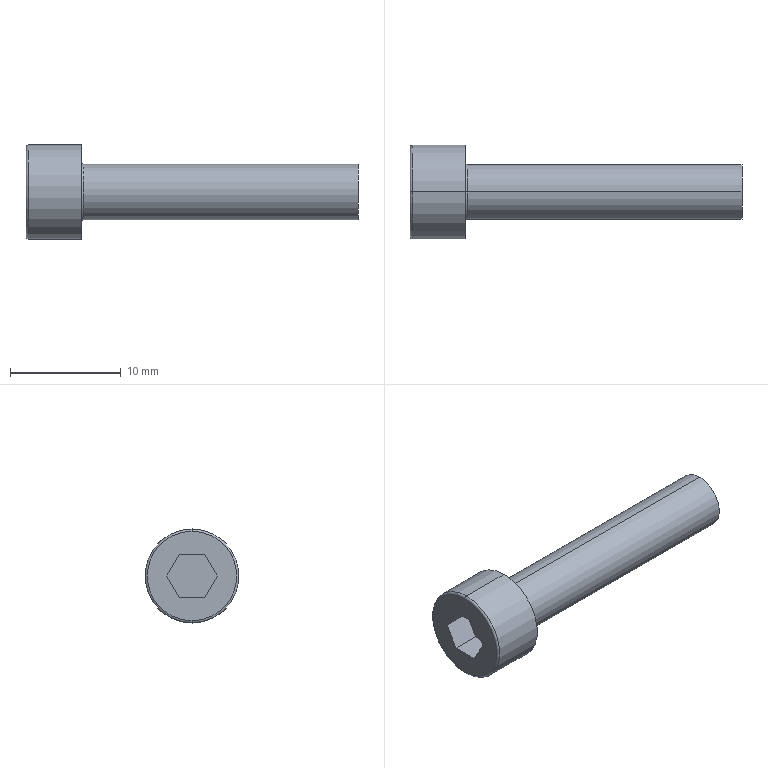Part | SolidWorks | features BlendCut 1, Cut 1, Fillet 1, LPattern 1, RevCut 1, Revolution 1 | 1 solid | 18 faces | box 30 x 8.5 x 8.5 mm | volume 740.448 mm3 | plane 10 | torus 4 | cylinder 4 | commonest cylinder face diameters 5 x2 8.5 x2
STEP:
#1=CARTESIAN_POINT('',(0.2,0.,-4.25));
#2=VERTEX_POINT('',#1);
#3=CARTESIAN_POINT('',(0.2,0.,4.25));
#4=VERTEX_POINT('',#3);
#5=CARTESIAN_POINT('',(0.2,0.,0.));
#6=DIRECTION('',(1.,0.,0.));
#7=DIRECTION('',(0.,0.,1.));
#8=AXIS2_PLACEMENT_3D('',#5,#6,#7);
#9=CIRCLE('',#8,4.25);
#10=EDGE_CURVE('',#2,#4,#9,.T.);
#11=ORIENTED_EDGE('',*,*,#10,.F.);
#12=CARTESIAN_POINT('',(0.,0.,-4.05));
#13=VERTEX_POINT('',#12);
#14=CARTESIAN_POINT('',(0.2,0.,-4.05));
#15=DIRECTION('',(0.,1.,0.));
#16=DIRECTION('',(0.,0.,1.));
#17=AXIS2_PLACEMENT_3D('',#14,#15,#16);
#18=CIRCLE('',#17,0.2);
#19=EDGE_CURVE('',#2,#13,#18,.T.);
#20=ORIENTED_EDGE('',*,*,#19,.T.);
#21=CARTESIAN_POINT('',(0.,0.,4.05));
#22=VERTEX_POINT('',#21);
#23=CARTESIAN_POINT('',(0.,0.,0.));
#24=DIRECTION('',(-1.,0.,0.));
#25=DIRECTION('',(0.,0.,1.));
#26=AXIS2_PLACEMENT_3D('',#23,#24,#25);
#27=CIRCLE('',#26,4.05);
#28=EDGE_CURVE('',#22,#13,#27,.T.);
#29=ORIENTED_EDGE('',*,*,#28,.F.);
#30=CARTESIAN_POINT('',(0.2,0.,4.05));
#31=DIRECTION('',(0.,-1.,0.));
#32=DIRECTION('',(0.,0.,-1.));
#33=AXIS2_PLACEMENT_3D('',#30,#31,#32);
#34=CIRCLE('',#33,0.2);
#35=EDGE_CURVE('',#4,#22,#34,.T.);
#36=ORIENTED_EDGE('',*,*,#35,.F.);
#37=EDGE_LOOP('',(#11,#20,#29,#36));
#38=FACE_OUTER_BOUND('',#37,.T.);
#39=CARTESIAN_POINT('',(0.2,0.,0.));
#40=DIRECTION('',(-1.,0.,0.));
#41=DIRECTION('',(0.,0.,1.));
#42=AXIS2_PLACEMENT_3D('',#39,#40,#41);
#43=TOROIDAL_SURFACE('',#42,4.05,0.2);
#44=ADVANCED_FACE('',(#38),#43,.T.);
#45=CARTESIAN_POINT('',(5.2,0.,-2.5));
#46=VERTEX_POINT('',#45);
#47=CARTESIAN_POINT('',(5.2,0.,2.5));
#48=VERTEX_POINT('',#47);
#49=CARTESIAN_POINT('',(5.2,0.,0.));
#50=DIRECTION('',(1.,0.,0.));
#51=DIRECTION('',(0.,0.,-1.));
#52=AXIS2_PLACEMENT_3D('',#49,#50,#51);
#53=CIRCLE('',#52,2.5);
#54=EDGE_CURVE('',#46,#48,#53,.T.);
#55=ORIENTED_EDGE('',*,*,#54,.T.);
#56=CARTESIAN_POINT('',(30.,0.,2.5));
#57=VERTEX_POINT('',#56);
#58=CARTESIAN_POINT('',(0.,0.,2.5));
#59=DIRECTION('',(1.,0.,0.));
#60=VECTOR('',#59,1000.);
#61=LINE('',#58,#60);
#62=EDGE_CURVE('',#48,#57,#61,.T.);
#63=ORIENTED_EDGE('',*,*,#62,.T.);
#64=CARTESIAN_POINT('',(30.,0.,-2.5));
#65=VERTEX_POINT('',#64);
#66=CARTESIAN_POINT('',(30.,0.,0.));
#67=DIRECTION('',(1.,0.,0.));
#68=DIRECTION('',(0.,0.,-1.));
#69=AXIS2_PLACEMENT_3D('',#66,#67,#68);
#70=CIRCLE('',#69,2.5);
#71=EDGE_CURVE('',#65,#57,#70,.T.);
#72=ORIENTED_EDGE('',*,*,#71,.F.);
#73=CARTESIAN_POINT('',(0.,0.,-2.5));
#74=DIRECTION('',(1.,0.,0.));
#75=VECTOR('',#74,1000.);
#76=LINE('',#73,#75);
#77=EDGE_CURVE('',#46,#65,#76,.T.);
#78=ORIENTED_EDGE('',*,*,#77,.F.);
#79=EDGE_LOOP('',(#55,#63,#72,#78));
#80=FACE_OUTER_BOUND('',#79,.T.);
#81=CARTESIAN_POINT('',(0.,0.,0.));
#82=DIRECTION('',(1.,0.,0.));
#83=DIRECTION('',(0.,0.,-1.));
#84=AXIS2_PLACEMENT_3D('',#81,#82,#83);
#85=CYLINDRICAL_SURFACE('',#84,2.5);
#86=ADVANCED_FACE('',(#80),#85,.T.);
#87=CARTESIAN_POINT('',(5.2,0.,0.));
#88=DIRECTION('',(1.,0.,0.));
#89=DIRECTION('',(0.,0.,-1.));
#90=AXIS2_PLACEMENT_3D('',#87,#88,#89);
#91=CIRCLE('',#90,2.5);
#92=EDGE_CURVE('',#48,#46,#91,.T.);
#93=ORIENTED_EDGE('',*,*,#92,.F.);
#94=CARTESIAN_POINT('',(5.,0.,2.7));
#95=VERTEX_POINT('',#94);
#96=CARTESIAN_POINT('',(5.2,0.,2.7));
#97=DIRECTION('',(0.,1.,0.));
#98=DIRECTION('',(0.,0.,1.));
#99=AXIS2_PLACEMENT_3D('',#96,#97,#98);
#100=CIRCLE('',#99,0.2);
#101=EDGE_CURVE('',#48,#95,#100,.T.);
#102=ORIENTED_EDGE('',*,*,#101,.T.);
#103=CARTESIAN_POINT('',(5.,0.,-2.7));
#104=VERTEX_POINT('',#103);
#105=CARTESIAN_POINT('',(5.,0.,0.));
#106=DIRECTION('',(1.,0.,0.));
#107=DIRECTION('',(0.,0.,-1.));
#108=AXIS2_PLACEMENT_3D('',#105,#106,#107);
#109=CIRCLE('',#108,2.7);
#110=EDGE_CURVE('',#95,#104,#109,.T.);
#111=ORIENTED_EDGE('',*,*,#110,.T.);
#112=CARTESIAN_POINT('',(5.2,0.,-2.7));
#113=DIRECTION('',(0.,-1.,0.));
#114=DIRECTION('',(0.,0.,-1.));
#115=AXIS2_PLACEMENT_3D('',#112,#113,#114);
#116=CIRCLE('',#115,0.2);
#117=EDGE_CURVE('',#46,#104,#116,.T.);
#118=ORIENTED_EDGE('',*,*,#117,.F.);
#119=EDGE_LOOP('',(#93,#102,#111,#118));
#120=FACE_OUTER_BOUND('',#119,.T.);
#121=CARTESIAN_POINT('',(5.2,0.,0.));
#122=DIRECTION('',(1.,0.,0.));
#123=DIRECTION('',(0.,0.,-1.));
#124=AXIS2_PLACEMENT_3D('',#121,#122,#123);
#125=TOROIDAL_SURFACE('',#124,2.7,0.2);
#126=ADVANCED_FACE('',(#120),#125,.F.);
#127=ORIENTED_EDGE('',*,*,#10,.T.);
#128=CARTESIAN_POINT('',(5.,0.,4.25));
#129=VERTEX_POINT('',#128);
#130=CARTESIAN_POINT('',(0.,0.,4.25));
#131=DIRECTION('',(1.,0.,0.));
#132=VECTOR('',#131,1000.);
#133=LINE('',#130,#132);
#134=EDGE_CURVE('',#4,#129,#133,.T.);
#135=ORIENTED_EDGE('',*,*,#134,.T.);
#136=CARTESIAN_POINT('',(5.,0.,-4.25));
#137=VERTEX_POINT('',#136);
#138=CARTESIAN_POINT('',(5.,0.,0.));
#139=DIRECTION('',(1.,0.,0.));
#140=DIRECTION('',(0.,0.,-1.));
#141=AXIS2_PLACEMENT_3D('',#138,#139,#140);
#142=CIRCLE('',#141,4.25);
#143=EDGE_CURVE('',#137,#129,#142,.T.);
#144=ORIENTED_EDGE('',*,*,#143,.F.);
#145=CARTESIAN_POINT('',(0.,0.,-4.25));
#146=DIRECTION('',(1.,0.,0.));
#147=VECTOR('',#146,1000.);
#148=LINE('',#145,#147);
#149=EDGE_CURVE('',#2,#137,#148,.T.);
#150=ORIENTED_EDGE('',*,*,#149,.F.);
#151=EDGE_LOOP('',(#127,#135,#144,#150));
#152=FACE_OUTER_BOUND('',#151,.T.);
#153=CARTESIAN_POINT('',(0.,0.,0.));
#154=DIRECTION('',(1.,0.,0.));
#155=DIRECTION('',(0.,0.,-1.));
#156=AXIS2_PLACEMENT_3D('',#153,#154,#155);
#157=CYLINDRICAL_SURFACE('',#156,4.25);
#158=ADVANCED_FACE('',(#152),#157,.T.);
#159=ORIENTED_EDGE('',*,*,#28,.T.);
#160=CARTESIAN_POINT('',(0.,0.,0.));
#161=DIRECTION('',(-1.,0.,0.));
#162=DIRECTION('',(0.,0.,1.));
#163=AXIS2_PLACEMENT_3D('',#160,#161,#162);
#164=CIRCLE('',#163,4.05);
#165=EDGE_CURVE('',#13,#22,#164,.T.);
#166=ORIENTED_EDGE('',*,*,#165,.T.);
#167=EDGE_LOOP('',(#159,#166));
#168=FACE_OUTER_BOUND('',#167,.T.);
#169=CARTESIAN_POINT('',(0.,-2.29,0.));
#170=VERTEX_POINT('',#169);
#171=CARTESIAN_POINT('',(0.,-1.145,1.983));
#172=VERTEX_POINT('',#171);
#173=CARTESIAN_POINT('',(0.,-2.29,0.));
#174=DIRECTION('',(0.,0.5,0.866));
#175=VECTOR('',#174,1000.);
#176=LINE('',#173,#175);
#177=EDGE_CURVE('',#170,#172,#176,.T.);
#178=ORIENTED_EDGE('',*,*,#177,.F.);
#179=CARTESIAN_POINT('',(0.,-1.145,-1.983));
#180=VERTEX_POINT('',#179);
#181=CARTESIAN_POINT('',(0.,-1.145,-1.983));
#182=DIRECTION('',(0.,-0.5,0.866));
#183=VECTOR('',#182,1000.);
#184=LINE('',#181,#183);
#185=EDGE_CURVE('',#180,#170,#184,.T.);
#186=ORIENTED_EDGE('',*,*,#185,.F.);
#187=CARTESIAN_POINT('',(0.,1.145,-1.983));
#188=VERTEX_POINT('',#187);
#189=CARTESIAN_POINT('',(0.,1.145,-1.983));
#190=DIRECTION('',(0.,-1.,0.));
#191=VECTOR('',#190,1000.);
#192=LINE('',#189,#191);
#193=EDGE_CURVE('',#188,#180,#192,.T.);
#194=ORIENTED_EDGE('',*,*,#193,.F.);
#195=CARTESIAN_POINT('',(0.,2.29,0.));
#196=VERTEX_POINT('',#195);
#197=CARTESIAN_POINT('',(0.,2.29,0.));
#198=DIRECTION('',(0.,-0.5,-0.866));
#199=VECTOR('',#198,1000.);
#200=LINE('',#197,#199);
#201=EDGE_CURVE('',#196,#188,#200,.T.);
#202=ORIENTED_EDGE('',*,*,#201,.F.);
#203=CARTESIAN_POINT('',(0.,1.145,1.983));
#204=VERTEX_POINT('',#203);
#205=CARTESIAN_POINT('',(0.,1.145,1.983));
#206=DIRECTION('',(0.,0.5,-0.866));
#207=VECTOR('',#206,1000.);
#208=LINE('',#205,#207);
#209=EDGE_CURVE('',#204,#196,#208,.T.);
#210=ORIENTED_EDGE('',*,*,#209,.F.);
#211=CARTESIAN_POINT('',(0.,-1.145,1.983));
#212=DIRECTION('',(0.,1.,0.));
#213=VECTOR('',#212,1000.);
#214=LINE('',#211,#213);
#215=EDGE_CURVE('',#172,#204,#214,.T.);
#216=ORIENTED_EDGE('',*,*,#215,.F.);
#217=EDGE_LOOP('',(#178,#186,#194,#202,#210,#216));
#218=FACE_BOUND('',#217,.T.);
#219=CARTESIAN_POINT('',(0.,0.,0.));
#220=DIRECTION('',(-1.,0.,0.));
#221=DIRECTION('',(0.,0.,1.));
#222=AXIS2_PLACEMENT_3D('',#219,#220,#221);
#223=PLANE('',#222);
#224=ADVANCED_FACE('',(#168,#218),#223,.T.);
#225=ORIENTED_EDGE('',*,*,#134,.F.);
#226=CARTESIAN_POINT('',(0.2,0.,0.));
#227=DIRECTION('',(1.,0.,0.));
#228=DIRECTION('',(0.,0.,1.));
#229=AXIS2_PLACEMENT_3D('',#226,#227,#228);
#230=CIRCLE('',#229,4.25);
#231=EDGE_CURVE('',#4,#2,#230,.T.);
#232=ORIENTED_EDGE('',*,*,#231,.T.);
#233=ORIENTED_EDGE('',*,*,#149,.T.);
#234=CARTESIAN_POINT('',(5.,0.,0.));
#235=DIRECTION('',(1.,0.,0.));
#236=DIRECTION('',(0.,0.,-1.));
#237=AXIS2_PLACEMENT_3D('',#234,#235,#236);
#238=CIRCLE('',#237,4.25);
#239=EDGE_CURVE('',#129,#137,#238,.T.);
#240=ORIENTED_EDGE('',*,*,#239,.F.);
#241=EDGE_LOOP('',(#225,#232,#233,#240));
#242=FACE_OUTER_BOUND('',#241,.T.);
#243=CARTESIAN_POINT('',(0.,0.,0.));
#244=DIRECTION('',(1.,0.,0.));
#245=DIRECTION('',(0.,0.,-1.));
#246=AXIS2_PLACEMENT_3D('',#243,#244,#245);
#247=CYLINDRICAL_SURFACE('',#246,4.25);
#248=ADVANCED_FACE('',(#242),#247,.T.);
#249=ORIENTED_EDGE('',*,*,#143,.T.);
#250=ORIENTED_EDGE('',*,*,#239,.T.);
#251=EDGE_LOOP('',(#249,#250));
#252=FACE_OUTER_BOUND('',#251,.T.);
#253=CARTESIAN_POINT('',(5.,0.,0.));
#254=DIRECTION('',(1.,0.,0.));
#255=DIRECTION('',(0.,0.,-1.));
#256=AXIS2_PLACEMENT_3D('',#253,#254,#255);
#257=CIRCLE('',#256,2.7);
#258=EDGE_CURVE('',#104,#95,#257,.T.);
#259=ORIENTED_EDGE('',*,*,#258,.F.);
#260=ORIENTED_EDGE('',*,*,#110,.F.);
#261=EDGE_LOOP('',(#259,#260));
#262=FACE_BOUND('',#261,.T.);
#263=CARTESIAN_POINT('',(5.,4.25,0.));
#264=DIRECTION('',(1.,0.,0.));
#265=DIRECTION('',(0.,0.,-1.));
#266=AXIS2_PLACEMENT_3D('',#263,#264,#265);
#267=PLANE('',#266);
#268=ADVANCED_FACE('',(#252,#262),#267,.T.);
#269=ORIENTED_EDGE('',*,*,#101,.F.);
#270=ORIENTED_EDGE('',*,*,#54,.F.);
#271=ORIENTED_EDGE('',*,*,#117,.T.);
#272=ORIENTED_EDGE('',*,*,#258,.T.);
#273=EDGE_LOOP('',(#269,#270,#271,#272));
#274=FACE_OUTER_BOUND('',#273,.T.);
#275=CARTESIAN_POINT('',(5.2,0.,0.));
#276=DIRECTION('',(1.,0.,0.));
#277=DIRECTION('',(0.,0.,-1.));
#278=AXIS2_PLACEMENT_3D('',#275,#276,#277);
#279=TOROIDAL_SURFACE('',#278,2.7,0.2);
#280=ADVANCED_FACE('',(#274),#279,.F.);
#281=ORIENTED_EDGE('',*,*,#62,.F.);
#282=ORIENTED_EDGE('',*,*,#92,.T.);
#283=ORIENTED_EDGE('',*,*,#77,.T.);
#284=CARTESIAN_POINT('',(30.,0.,0.));
#285=DIRECTION('',(1.,0.,0.));
#286=DIRECTION('',(0.,0.,-1.));
#287=AXIS2_PLACEMENT_3D('',#284,#285,#286);
#288=CIRCLE('',#287,2.5);
#289=EDGE_CURVE('',#57,#65,#288,.T.);
#290=ORIENTED_EDGE('',*,*,#289,.F.);
#291=EDGE_LOOP('',(#281,#282,#283,#290));
#292=FACE_OUTER_BOUND('',#291,.T.);
#293=CARTESIAN_POINT('',(0.,0.,0.));
#294=DIRECTION('',(1.,0.,0.));
#295=DIRECTION('',(0.,0.,-1.));
#296=AXIS2_PLACEMENT_3D('',#293,#294,#295);
#297=CYLINDRICAL_SURFACE('',#296,2.5);
#298=ADVANCED_FACE('',(#292),#297,.T.);
#299=ORIENTED_EDGE('',*,*,#71,.T.);
#300=ORIENTED_EDGE('',*,*,#289,.T.);
#301=EDGE_LOOP('',(#299,#300));
#302=FACE_OUTER_BOUND('',#301,.T.);
#303=CARTESIAN_POINT('',(30.,2.5,0.));
#304=DIRECTION('',(1.,0.,0.));
#305=DIRECTION('',(0.,0.,-1.));
#306=AXIS2_PLACEMENT_3D('',#303,#304,#305);
#307=PLANE('',#306);
#308=ADVANCED_FACE('',(#302),#307,.T.);
#309=ORIENTED_EDGE('',*,*,#177,.T.);
#310=CARTESIAN_POINT('',(2.5,-1.145,1.983));
#311=VERTEX_POINT('',#310);
#312=CARTESIAN_POINT('',(2.5,-1.145,1.983));
#313=DIRECTION('',(-1.,0.,0.));
#314=VECTOR('',#313,1000.);
#315=LINE('',#312,#314);
#316=EDGE_CURVE('',#311,#172,#315,.T.);
#317=ORIENTED_EDGE('',*,*,#316,.F.);
#318=CARTESIAN_POINT('',(2.5,-2.29,0.));
#319=VERTEX_POINT('',#318);
#320=CARTESIAN_POINT('',(2.5,-2.29,0.));
#321=DIRECTION('',(0.,0.5,0.866));
#322=VECTOR('',#321,1000.);
#323=LINE('',#320,#322);
#324=EDGE_CURVE('',#319,#311,#323,.T.);
#325=ORIENTED_EDGE('',*,*,#324,.F.);
#326=CARTESIAN_POINT('',(2.5,-2.29,0.));
#327=DIRECTION('',(-1.,0.,0.));
#328=VECTOR('',#327,1000.);
#329=LINE('',#326,#328);
#330=EDGE_CURVE('',#319,#170,#329,.T.);
#331=ORIENTED_EDGE('',*,*,#330,.T.);
#332=EDGE_LOOP('',(#309,#317,#325,#331));
#333=FACE_OUTER_BOUND('',#332,.T.);
#334=CARTESIAN_POINT('',(2.5,-2.29,0.));
#335=DIRECTION('',(0.,-0.866,0.5));
#336=DIRECTION('',(0.,-0.5,-0.866));
#337=AXIS2_PLACEMENT_3D('',#334,#335,#336);
#338=PLANE('',#337);
#339=ADVANCED_FACE('',(#333),#338,.F.);
#340=ORIENTED_EDGE('',*,*,#185,.T.);
#341=ORIENTED_EDGE('',*,*,#330,.F.);
#342=CARTESIAN_POINT('',(2.5,-1.145,-1.983));
#343=VERTEX_POINT('',#342);
#344=CARTESIAN_POINT('',(2.5,-1.145,-1.983));
#345=DIRECTION('',(0.,-0.5,0.866));
#346=VECTOR('',#345,1000.);
#347=LINE('',#344,#346);
#348=EDGE_CURVE('',#343,#319,#347,.T.);
#349=ORIENTED_EDGE('',*,*,#348,.F.);
#350=CARTESIAN_POINT('',(2.5,-1.145,-1.983));
#351=DIRECTION('',(-1.,0.,0.));
#352=VECTOR('',#351,1000.);
#353=LINE('',#350,#352);
#354=EDGE_CURVE('',#343,#180,#353,.T.);
#355=ORIENTED_EDGE('',*,*,#354,.T.);
#356=EDGE_LOOP('',(#340,#341,#349,#355));
#357=FACE_OUTER_BOUND('',#356,.T.);
#358=CARTESIAN_POINT('',(2.5,-1.145,-1.983));
#359=DIRECTION('',(0.,-0.866,-0.5));
#360=DIRECTION('',(0.,0.5,-0.866));
#361=AXIS2_PLACEMENT_3D('',#358,#359,#360);
#362=PLANE('',#361);
#363=ADVANCED_FACE('',(#357),#362,.F.);
#364=ORIENTED_EDGE('',*,*,#193,.T.);
#365=ORIENTED_EDGE('',*,*,#354,.F.);
#366=CARTESIAN_POINT('',(2.5,1.145,-1.983));
#367=VERTEX_POINT('',#366);
#368=CARTESIAN_POINT('',(2.5,1.145,-1.983));
#369=DIRECTION('',(0.,-1.,0.));
#370=VECTOR('',#369,1000.);
#371=LINE('',#368,#370);
#372=EDGE_CURVE('',#367,#343,#371,.T.);
#373=ORIENTED_EDGE('',*,*,#372,.F.);
#374=CARTESIAN_POINT('',(2.5,1.145,-1.983));
#375=DIRECTION('',(-1.,0.,0.));
#376=VECTOR('',#375,1000.);
#377=LINE('',#374,#376);
#378=EDGE_CURVE('',#367,#188,#377,.T.);
#379=ORIENTED_EDGE('',*,*,#378,.T.);
#380=EDGE_LOOP('',(#364,#365,#373,#379));
#381=FACE_OUTER_BOUND('',#380,.T.);
#382=CARTESIAN_POINT('',(2.5,1.145,-1.983));
#383=DIRECTION('',(0.,0.,-1.));
#384=DIRECTION('',(0.,1.,0.));
#385=AXIS2_PLACEMENT_3D('',#382,#383,#384);
#386=PLANE('',#385);
#387=ADVANCED_FACE('',(#381),#386,.F.);
#388=ORIENTED_EDGE('',*,*,#201,.T.);
#389=ORIENTED_EDGE('',*,*,#378,.F.);
#390=CARTESIAN_POINT('',(2.5,2.29,0.));
#391=VERTEX_POINT('',#390);
#392=CARTESIAN_POINT('',(2.5,2.29,0.));
#393=DIRECTION('',(0.,-0.5,-0.866));
#394=VECTOR('',#393,1000.);
#395=LINE('',#392,#394);
#396=EDGE_CURVE('',#391,#367,#395,.T.);
#397=ORIENTED_EDGE('',*,*,#396,.F.);
#398=CARTESIAN_POINT('',(2.5,2.29,0.));
#399=DIRECTION('',(-1.,0.,0.));
#400=VECTOR('',#399,1000.);
#401=LINE('',#398,#400);
#402=EDGE_CURVE('',#391,#196,#401,.T.);
#403=ORIENTED_EDGE('',*,*,#402,.T.);
#404=EDGE_LOOP('',(#388,#389,#397,#403));
#405=FACE_OUTER_BOUND('',#404,.T.);
#406=CARTESIAN_POINT('',(2.5,2.29,0.));
#407=DIRECTION('',(0.,0.866,-0.5));
#408=DIRECTION('',(0.,0.5,0.866));
#409=AXIS2_PLACEMENT_3D('',#406,#407,#408);
#410=PLANE('',#409);
#411=ADVANCED_FACE('',(#405),#410,.F.);
#412=ORIENTED_EDGE('',*,*,#209,.T.);
#413=ORIENTED_EDGE('',*,*,#402,.F.);
#414=CARTESIAN_POINT('',(2.5,1.145,1.983));
#415=VERTEX_POINT('',#414);
#416=CARTESIAN_POINT('',(2.5,1.145,1.983));
#417=DIRECTION('',(0.,0.5,-0.866));
#418=VECTOR('',#417,1000.);
#419=LINE('',#416,#418);
#420=EDGE_CURVE('',#415,#391,#419,.T.);
#421=ORIENTED_EDGE('',*,*,#420,.F.);
#422=CARTESIAN_POINT('',(2.5,1.145,1.983));
#423=DIRECTION('',(-1.,0.,0.));
#424=VECTOR('',#423,1000.);
#425=LINE('',#422,#424);
#426=EDGE_CURVE('',#415,#204,#425,.T.);
#427=ORIENTED_EDGE('',*,*,#426,.T.);
#428=EDGE_LOOP('',(#412,#413,#421,#427));
#429=FACE_OUTER_BOUND('',#428,.T.);
#430=CARTESIAN_POINT('',(2.5,1.145,1.983));
#431=DIRECTION('',(0.,0.866,0.5));
#432=DIRECTION('',(0.,-0.5,0.866));
#433=AXIS2_PLACEMENT_3D('',#430,#431,#432);
#434=PLANE('',#433);
#435=ADVANCED_FACE('',(#429),#434,.F.);
#436=ORIENTED_EDGE('',*,*,#215,.T.);
#437=ORIENTED_EDGE('',*,*,#426,.F.);
#438=CARTESIAN_POINT('',(2.5,-1.145,1.983));
#439=DIRECTION('',(0.,1.,0.));
#440=VECTOR('',#439,1000.);
#441=LINE('',#438,#440);
#442=EDGE_CURVE('',#311,#415,#441,.T.);
#443=ORIENTED_EDGE('',*,*,#442,.F.);
#444=ORIENTED_EDGE('',*,*,#316,.T.);
#445=EDGE_LOOP('',(#436,#437,#443,#444));
#446=FACE_OUTER_BOUND('',#445,.T.);
#447=CARTESIAN_POINT('',(2.5,-1.145,1.983));
#448=DIRECTION('',(0.,0.,1.));
#449=DIRECTION('',(0.,-1.,0.));
#450=AXIS2_PLACEMENT_3D('',#447,#448,#449);
#451=PLANE('',#450);
#452=ADVANCED_FACE('',(#446),#451,.F.);
#453=ORIENTED_EDGE('',*,*,#324,.T.);
#454=ORIENTED_EDGE('',*,*,#442,.T.);
#455=ORIENTED_EDGE('',*,*,#420,.T.);
#456=ORIENTED_EDGE('',*,*,#396,.T.);
#457=ORIENTED_EDGE('',*,*,#372,.T.);
#458=ORIENTED_EDGE('',*,*,#348,.T.);
#459=EDGE_LOOP('',(#453,#454,#455,#456,#457,#458));
#460=FACE_OUTER_BOUND('',#459,.T.);
#461=CARTESIAN_POINT('',(2.5,-1.145,1.983));
#462=DIRECTION('',(-1.,0.,0.));
#463=DIRECTION('',(0.,0.,1.));
#464=AXIS2_PLACEMENT_3D('',#461,#462,#463);
#465=PLANE('',#464);
#466=ADVANCED_FACE('',(#460),#465,.T.);
#467=ORIENTED_EDGE('',*,*,#19,.F.);
#468=ORIENTED_EDGE('',*,*,#231,.F.);
#469=ORIENTED_EDGE('',*,*,#35,.T.);
#470=ORIENTED_EDGE('',*,*,#165,.F.);
#471=EDGE_LOOP('',(#467,#468,#469,#470));
#472=FACE_OUTER_BOUND('',#471,.T.);
#473=CARTESIAN_POINT('',(0.2,0.,0.));
#474=DIRECTION('',(-1.,0.,0.));
#475=DIRECTION('',(0.,0.,1.));
#476=AXIS2_PLACEMENT_3D('',#473,#474,#475);
#477=TOROIDAL_SURFACE('',#476,4.05,0.2);
#478=ADVANCED_FACE('',(#472),#477,.T.);
#479=CLOSED_SHELL('',(#44,#86,#126,#158,#224,#248,#268,#280,#298,#308,#339,#363,#387,#411,#435,#452,#466,#478));
#480=MANIFOLD_SOLID_BREP('',#479);
#481=CARTESIAN_POINT('',(0.,0.,0.));
#482=DIRECTION('',(0.,0.,1.));
#483=DIRECTION('',(1.,0.,0.));
#484=AXIS2_PLACEMENT_3D('',#481,#482,#483);
#485=(LENGTH_UNIT()NAMED_UNIT(*)SI_UNIT(.MILLI.,.METRE.));
#486=UNCERTAINTY_MEASURE_WITH_UNIT(LENGTH_MEASURE(0.00001),#485,'','');
#487=(NAMED_UNIT(*)PLANE_ANGLE_UNIT()SI_UNIT($,.RADIAN.));
#488=(NAMED_UNIT(*)SI_UNIT($,.STERADIAN.)SOLID_ANGLE_UNIT());
#489=(GEOMETRIC_REPRESENTATION_CONTEXT(3)GLOBAL_UNCERTAINTY_ASSIGNED_CONTEXT((#486))GLOBAL_UNIT_ASSIGNED_CONTEXT((#485,#487,#488))REPRESENTATION_CONTEXT('',''));
#490=ADVANCED_BREP_SHAPE_REPRESENTATION('',(#480,#484),#489);